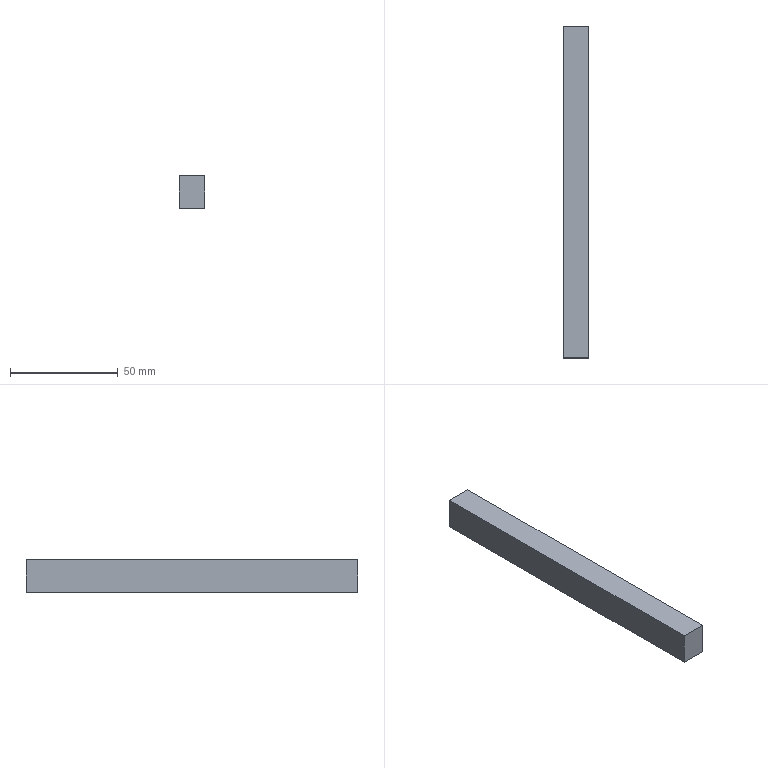Part | NX | features solid 2 | 1 solid | 6 faces | box 12 x 154 x 15 mm | volume 27720 mm3 | plane 6
STEP:
#1=CARTESIAN_POINT('',(-903.,-226.5,-20.));
#2=VERTEX_POINT('',#1);
#3=CARTESIAN_POINT('',(-903.,-226.5,-35.));
#4=VERTEX_POINT('',#3);
#5=CARTESIAN_POINT('',(-903.,-226.5,-35.));
#6=DIRECTION('',(0.,0.,1.));
#7=VECTOR('',#6,1000.);
#8=LINE('',#5,#7);
#9=EDGE_CURVE('',#2,#4,#8,.F.);
#10=ORIENTED_EDGE('',*,*,#9,.F.);
#11=CARTESIAN_POINT('',(-915.,-226.5,-20.));
#12=VERTEX_POINT('',#11);
#13=CARTESIAN_POINT('',(-932.,-226.5,-20.));
#14=DIRECTION('',(1.,0.,0.));
#15=VECTOR('',#14,1000.);
#16=LINE('',#13,#15);
#17=EDGE_CURVE('',#12,#2,#16,.T.);
#18=ORIENTED_EDGE('',*,*,#17,.F.);
#19=CARTESIAN_POINT('',(-915.,-226.5,-35.));
#20=VERTEX_POINT('',#19);
#21=CARTESIAN_POINT('',(-915.,-226.5,-35.));
#22=DIRECTION('',(0.,0.,1.));
#23=VECTOR('',#22,1000.);
#24=LINE('',#21,#23);
#25=EDGE_CURVE('',#20,#12,#24,.T.);
#26=ORIENTED_EDGE('',*,*,#25,.F.);
#27=CARTESIAN_POINT('',(-932.,-226.5,-35.));
#28=DIRECTION('',(1.,0.,0.));
#29=VECTOR('',#28,1000.);
#30=LINE('',#27,#29);
#31=EDGE_CURVE('',#20,#4,#30,.T.);
#32=ORIENTED_EDGE('',*,*,#31,.T.);
#33=EDGE_LOOP('',(#10,#18,#26,#32));
#34=FACE_BOUND('',#33,.T.);
#35=CARTESIAN_POINT('',(-903.,-226.5,-20.));
#36=DIRECTION('',(0.,-1.,0.));
#37=DIRECTION('',(0.,0.,-1.));
#38=AXIS2_PLACEMENT_3D('',#35,#36,#37);
#39=PLANE('',#38);
#40=ADVANCED_FACE('',(#34),#39,.T.);
#41=CARTESIAN_POINT('',(-903.,-72.5,-35.));
#42=VERTEX_POINT('',#41);
#43=CARTESIAN_POINT('',(-915.,-72.5,-35.));
#44=VERTEX_POINT('',#43);
#45=CARTESIAN_POINT('',(-932.,-72.5,-35.));
#46=DIRECTION('',(-1.,0.,0.));
#47=VECTOR('',#46,1000.);
#48=LINE('',#45,#47);
#49=EDGE_CURVE('',#42,#44,#48,.T.);
#50=ORIENTED_EDGE('',*,*,#49,.T.);
#51=CARTESIAN_POINT('',(-915.,-72.5,-20.));
#52=VERTEX_POINT('',#51);
#53=CARTESIAN_POINT('',(-915.,-72.5,-20.));
#54=DIRECTION('',(0.,0.,1.));
#55=VECTOR('',#54,1000.);
#56=LINE('',#53,#55);
#57=EDGE_CURVE('',#44,#52,#56,.T.);
#58=ORIENTED_EDGE('',*,*,#57,.T.);
#59=CARTESIAN_POINT('',(-903.,-72.5,-20.));
#60=VERTEX_POINT('',#59);
#61=CARTESIAN_POINT('',(-932.,-72.5,-20.));
#62=DIRECTION('',(-1.,0.,0.));
#63=VECTOR('',#62,1000.);
#64=LINE('',#61,#63);
#65=EDGE_CURVE('',#60,#52,#64,.T.);
#66=ORIENTED_EDGE('',*,*,#65,.F.);
#67=CARTESIAN_POINT('',(-903.,-72.5,-35.));
#68=DIRECTION('',(0.,0.,-1.));
#69=VECTOR('',#68,1000.);
#70=LINE('',#67,#69);
#71=EDGE_CURVE('',#42,#60,#70,.F.);
#72=ORIENTED_EDGE('',*,*,#71,.F.);
#73=EDGE_LOOP('',(#50,#58,#66,#72));
#74=FACE_BOUND('',#73,.T.);
#75=CARTESIAN_POINT('',(-915.,-72.5,-20.));
#76=DIRECTION('',(0.,1.,0.));
#77=DIRECTION('',(0.,0.,1.));
#78=AXIS2_PLACEMENT_3D('',#75,#76,#77);
#79=PLANE('',#78);
#80=ADVANCED_FACE('',(#74),#79,.T.);
#81=CARTESIAN_POINT('',(-903.,-226.5,-20.));
#82=DIRECTION('',(0.,1.,0.));
#83=VECTOR('',#82,1000.);
#84=LINE('',#81,#83);
#85=EDGE_CURVE('',#2,#60,#84,.T.);
#86=ORIENTED_EDGE('',*,*,#85,.F.);
#87=ORIENTED_EDGE('',*,*,#9,.T.);
#88=CARTESIAN_POINT('',(-903.,-226.5,-35.));
#89=DIRECTION('',(0.,1.,0.));
#90=VECTOR('',#89,1000.);
#91=LINE('',#88,#90);
#92=EDGE_CURVE('',#4,#42,#91,.T.);
#93=ORIENTED_EDGE('',*,*,#92,.T.);
#94=ORIENTED_EDGE('',*,*,#71,.T.);
#95=EDGE_LOOP('',(#86,#87,#93,#94));
#96=FACE_BOUND('',#95,.T.);
#97=CARTESIAN_POINT('',(-903.,-226.5,-35.));
#98=DIRECTION('',(-1.,0.,0.));
#99=DIRECTION('',(0.,0.,1.));
#100=AXIS2_PLACEMENT_3D('',#97,#98,#99);
#101=PLANE('',#100);
#102=ADVANCED_FACE('',(#96),#101,.F.);
#103=CARTESIAN_POINT('',(-915.,-226.5,-35.));
#104=DIRECTION('',(0.,1.,0.));
#105=VECTOR('',#104,1000.);
#106=LINE('',#103,#105);
#107=EDGE_CURVE('',#20,#44,#106,.T.);
#108=ORIENTED_EDGE('',*,*,#107,.F.);
#109=ORIENTED_EDGE('',*,*,#25,.T.);
#110=CARTESIAN_POINT('',(-915.,-226.5,-20.));
#111=DIRECTION('',(0.,1.,0.));
#112=VECTOR('',#111,1000.);
#113=LINE('',#110,#112);
#114=EDGE_CURVE('',#12,#52,#113,.T.);
#115=ORIENTED_EDGE('',*,*,#114,.T.);
#116=ORIENTED_EDGE('',*,*,#57,.F.);
#117=EDGE_LOOP('',(#108,#109,#115,#116));
#118=FACE_BOUND('',#117,.T.);
#119=CARTESIAN_POINT('',(-915.,-226.5,-35.));
#120=DIRECTION('',(-1.,0.,0.));
#121=DIRECTION('',(0.,0.,1.));
#122=AXIS2_PLACEMENT_3D('',#119,#120,#121);
#123=PLANE('',#122);
#124=ADVANCED_FACE('',(#118),#123,.T.);
#125=ORIENTED_EDGE('',*,*,#31,.F.);
#126=ORIENTED_EDGE('',*,*,#107,.T.);
#127=ORIENTED_EDGE('',*,*,#49,.F.);
#128=ORIENTED_EDGE('',*,*,#92,.F.);
#129=EDGE_LOOP('',(#125,#126,#127,#128));
#130=FACE_BOUND('',#129,.T.);
#131=CARTESIAN_POINT('',(-932.,-124.5,-35.));
#132=DIRECTION('',(0.,0.,1.));
#133=DIRECTION('',(1.,0.,0.));
#134=AXIS2_PLACEMENT_3D('',#131,#132,#133);
#135=PLANE('',#134);
#136=ADVANCED_FACE('',(#130),#135,.F.);
#137=ORIENTED_EDGE('',*,*,#114,.F.);
#138=ORIENTED_EDGE('',*,*,#17,.T.);
#139=ORIENTED_EDGE('',*,*,#85,.T.);
#140=ORIENTED_EDGE('',*,*,#65,.T.);
#141=EDGE_LOOP('',(#137,#138,#139,#140));
#142=FACE_BOUND('',#141,.T.);
#143=CARTESIAN_POINT('',(-932.,-124.5,-20.));
#144=DIRECTION('',(0.,0.,1.));
#145=DIRECTION('',(1.,0.,0.));
#146=AXIS2_PLACEMENT_3D('',#143,#144,#145);
#147=PLANE('',#146);
#148=ADVANCED_FACE('',(#142),#147,.T.);
#149=CLOSED_SHELL('',(#40,#80,#102,#124,#136,#148));
#150=MANIFOLD_SOLID_BREP('',#149);
#151=(LENGTH_UNIT()NAMED_UNIT(*)SI_UNIT(.MILLI.,.METRE.));
#152=UNCERTAINTY_MEASURE_WITH_UNIT(LENGTH_MEASURE(0.00001),#151,'','');
#153=(NAMED_UNIT(*)PLANE_ANGLE_UNIT()SI_UNIT($,.RADIAN.));
#154=(NAMED_UNIT(*)SI_UNIT($,.STERADIAN.)SOLID_ANGLE_UNIT());
#155=(GEOMETRIC_REPRESENTATION_CONTEXT(3)GLOBAL_UNCERTAINTY_ASSIGNED_CONTEXT((#152))GLOBAL_UNIT_ASSIGNED_CONTEXT((#151,#153,#154))REPRESENTATION_CONTEXT('',''));
#156=ADVANCED_BREP_SHAPE_REPRESENTATION('',(#150),#155);